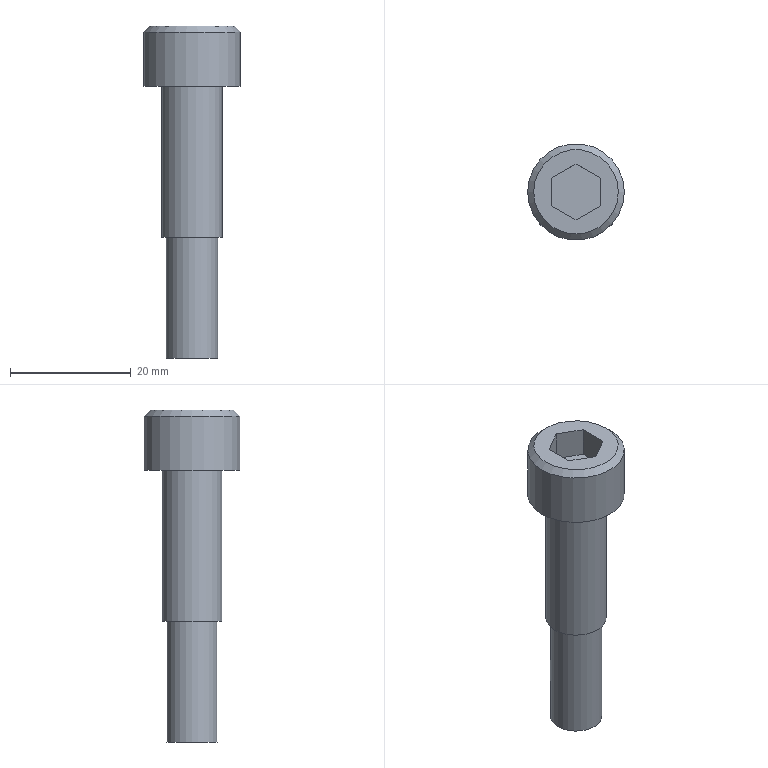Part | STEP file | M3-10_id42_x_t | 1 solid | 15 faces | box 16 x 16 x 55 mm | volume 4808 mm3 | plane 11 | cylinder 3 | cone 1 | commonest cylinder face diameters 8.5 x1 10 x1 16 x1
STEP:
#1=CARTESIAN_POINT('',(-209.8,-31.,-47.));
#2=VERTEX_POINT('',#1);
#3=CARTESIAN_POINT('',(-205.55,-31.,-47.));
#4=DIRECTION('',(0.,0.,-1.));
#5=DIRECTION('',(-1.,0.,0.));
#6=AXIS2_PLACEMENT_3D('',#3,#4,#5);
#7=CIRCLE('',#6,4.25);
#8=EDGE_CURVE('',#2,#2,#7,.T.);
#9=ORIENTED_EDGE('',*,*,#8,.F.);
#10=EDGE_LOOP('',(#9));
#11=FACE_BOUND('',#10,.T.);
#12=CARTESIAN_POINT('',(-200.55,-31.,-47.));
#13=VERTEX_POINT('',#12);
#14=CARTESIAN_POINT('',(-205.55,-31.,-47.));
#15=DIRECTION('',(0.,0.,1.));
#16=DIRECTION('',(1.,0.,0.));
#17=AXIS2_PLACEMENT_3D('',#14,#15,#16);
#18=CIRCLE('',#17,5.);
#19=EDGE_CURVE('',#13,#13,#18,.T.);
#20=ORIENTED_EDGE('',*,*,#19,.F.);
#21=EDGE_LOOP('',(#20));
#22=FACE_BOUND('',#21,.T.);
#23=CARTESIAN_POINT('',(-205.55,-31.,-47.));
#24=DIRECTION('',(0.,0.,-1.));
#25=DIRECTION('',(-1.,0.,0.));
#26=AXIS2_PLACEMENT_3D('',#23,#24,#25);
#27=PLANE('',#26);
#28=ADVANCED_FACE('',(#11,#22),#27,.T.);
#29=CARTESIAN_POINT('',(-210.55,-31.,-22.));
#30=VERTEX_POINT('',#29);
#31=CARTESIAN_POINT('',(-205.55,-31.,-22.));
#32=DIRECTION('',(0.,0.,1.));
#33=DIRECTION('',(-1.,0.,0.));
#34=AXIS2_PLACEMENT_3D('',#31,#32,#33);
#35=CIRCLE('',#34,5.);
#36=EDGE_CURVE('',#30,#30,#35,.T.);
#37=ORIENTED_EDGE('',*,*,#36,.F.);
#38=EDGE_LOOP('',(#37));
#39=FACE_BOUND('',#38,.T.);
#40=ORIENTED_EDGE('',*,*,#19,.T.);
#41=EDGE_LOOP('',(#40));
#42=FACE_BOUND('',#41,.T.);
#43=CARTESIAN_POINT('',(-205.55,-31.,-47.));
#44=DIRECTION('',(0.,0.,1.));
#45=DIRECTION('',(1.,0.,0.));
#46=AXIS2_PLACEMENT_3D('',#43,#44,#45);
#47=CYLINDRICAL_SURFACE('',#46,5.);
#48=ADVANCED_FACE('',(#39,#42),#47,.T.);
#49=CARTESIAN_POINT('',(-201.3,-31.,-67.));
#50=VERTEX_POINT('',#49);
#51=CARTESIAN_POINT('',(-205.55,-31.,-67.));
#52=DIRECTION('',(0.,0.,1.));
#53=DIRECTION('',(1.,0.,0.));
#54=AXIS2_PLACEMENT_3D('',#51,#52,#53);
#55=CIRCLE('',#54,4.25);
#56=EDGE_CURVE('',#50,#50,#55,.T.);
#57=ORIENTED_EDGE('',*,*,#56,.F.);
#58=EDGE_LOOP('',(#57));
#59=FACE_OUTER_BOUND('',#58,.T.);
#60=CARTESIAN_POINT('',(-205.55,-31.,-67.));
#61=DIRECTION('',(0.,0.,-1.));
#62=DIRECTION('',(-1.,0.,0.));
#63=AXIS2_PLACEMENT_3D('',#60,#61,#62);
#64=PLANE('',#63);
#65=ADVANCED_FACE('',(#59),#64,.T.);
#66=ORIENTED_EDGE('',*,*,#56,.T.);
#67=EDGE_LOOP('',(#66));
#68=FACE_BOUND('',#67,.T.);
#69=ORIENTED_EDGE('',*,*,#8,.T.);
#70=EDGE_LOOP('',(#69));
#71=FACE_BOUND('',#70,.T.);
#72=CARTESIAN_POINT('',(-205.55,-31.,-47.));
#73=DIRECTION('',(0.,0.,-1.));
#74=DIRECTION('',(1.,0.,0.));
#75=AXIS2_PLACEMENT_3D('',#72,#73,#74);
#76=CYLINDRICAL_SURFACE('',#75,4.25);
#77=ADVANCED_FACE('',(#68,#71),#76,.T.);
#78=CARTESIAN_POINT('',(-209.55,-28.691,-12.));
#79=VERTEX_POINT('',#78);
#80=CARTESIAN_POINT('',(-209.55,-33.309,-12.));
#81=VERTEX_POINT('',#80);
#82=CARTESIAN_POINT('',(-209.55,-28.691,-12.));
#83=DIRECTION('',(0.,-1.,0.));
#84=VECTOR('',#83,1.);
#85=LINE('',#82,#84);
#86=EDGE_CURVE('',#79,#81,#85,.T.);
#87=ORIENTED_EDGE('',*,*,#86,.F.);
#88=CARTESIAN_POINT('',(-205.55,-26.381,-12.));
#89=VERTEX_POINT('',#88);
#90=CARTESIAN_POINT('',(-205.55,-26.381,-12.));
#91=DIRECTION('',(-0.866,-0.5,0.));
#92=VECTOR('',#91,1.);
#93=LINE('',#90,#92);
#94=EDGE_CURVE('',#89,#79,#93,.T.);
#95=ORIENTED_EDGE('',*,*,#94,.F.);
#96=CARTESIAN_POINT('',(-201.55,-28.691,-12.));
#97=VERTEX_POINT('',#96);
#98=CARTESIAN_POINT('',(-201.55,-28.691,-12.));
#99=DIRECTION('',(-0.866,0.5,0.));
#100=VECTOR('',#99,1.);
#101=LINE('',#98,#100);
#102=EDGE_CURVE('',#97,#89,#101,.T.);
#103=ORIENTED_EDGE('',*,*,#102,.F.);
#104=CARTESIAN_POINT('',(-201.55,-33.309,-12.));
#105=VERTEX_POINT('',#104);
#106=CARTESIAN_POINT('',(-201.55,-33.309,-12.));
#107=DIRECTION('',(0.,1.,0.));
#108=VECTOR('',#107,1.);
#109=LINE('',#106,#108);
#110=EDGE_CURVE('',#105,#97,#109,.T.);
#111=ORIENTED_EDGE('',*,*,#110,.F.);
#112=CARTESIAN_POINT('',(-205.55,-35.619,-12.));
#113=VERTEX_POINT('',#112);
#114=CARTESIAN_POINT('',(-205.55,-35.619,-12.));
#115=DIRECTION('',(0.866,0.5,0.));
#116=VECTOR('',#115,1.);
#117=LINE('',#114,#116);
#118=EDGE_CURVE('',#113,#105,#117,.T.);
#119=ORIENTED_EDGE('',*,*,#118,.F.);
#120=CARTESIAN_POINT('',(-209.55,-33.309,-12.));
#121=DIRECTION('',(0.866,-0.5,0.));
#122=VECTOR('',#121,1.);
#123=LINE('',#120,#122);
#124=EDGE_CURVE('',#81,#113,#123,.T.);
#125=ORIENTED_EDGE('',*,*,#124,.F.);
#126=EDGE_LOOP('',(#87,#95,#103,#111,#119,#125));
#127=FACE_BOUND('',#126,.T.);
#128=CARTESIAN_POINT('',(-198.55,-31.,-12.));
#129=VERTEX_POINT('',#128);
#130=CARTESIAN_POINT('',(-205.55,-31.,-12.));
#131=DIRECTION('',(0.,0.,1.));
#132=DIRECTION('',(1.,0.,0.));
#133=AXIS2_PLACEMENT_3D('',#130,#131,#132);
#134=CIRCLE('',#133,7.);
#135=EDGE_CURVE('',#129,#129,#134,.T.);
#136=ORIENTED_EDGE('',*,*,#135,.T.);
#137=EDGE_LOOP('',(#136));
#138=FACE_BOUND('',#137,.T.);
#139=CARTESIAN_POINT('',(-205.55,-31.,-12.));
#140=DIRECTION('',(0.,0.,1.));
#141=DIRECTION('',(1.,0.,0.));
#142=AXIS2_PLACEMENT_3D('',#139,#140,#141);
#143=PLANE('',#142);
#144=ADVANCED_FACE('',(#127,#138),#143,.T.);
#145=ORIENTED_EDGE('',*,*,#36,.T.);
#146=EDGE_LOOP('',(#145));
#147=FACE_BOUND('',#146,.T.);
#148=CARTESIAN_POINT('',(-197.55,-31.,-22.));
#149=VERTEX_POINT('',#148);
#150=CARTESIAN_POINT('',(-205.55,-31.,-22.));
#151=DIRECTION('',(0.,0.,1.));
#152=DIRECTION('',(1.,0.,0.));
#153=AXIS2_PLACEMENT_3D('',#150,#151,#152);
#154=CIRCLE('',#153,8.);
#155=EDGE_CURVE('',#149,#149,#154,.T.);
#156=ORIENTED_EDGE('',*,*,#155,.F.);
#157=EDGE_LOOP('',(#156));
#158=FACE_BOUND('',#157,.T.);
#159=CARTESIAN_POINT('',(-205.55,-31.,-22.));
#160=DIRECTION('',(0.,0.,-1.));
#161=DIRECTION('',(-1.,0.,0.));
#162=AXIS2_PLACEMENT_3D('',#159,#160,#161);
#163=PLANE('',#162);
#164=ADVANCED_FACE('',(#147,#158),#163,.T.);
#165=CARTESIAN_POINT('',(-197.55,-31.,-13.));
#166=VERTEX_POINT('',#165);
#167=CARTESIAN_POINT('',(-205.55,-31.,-13.));
#168=DIRECTION('',(0.,0.,-1.));
#169=DIRECTION('',(1.,0.,0.));
#170=AXIS2_PLACEMENT_3D('',#167,#168,#169);
#171=CIRCLE('',#170,8.);
#172=EDGE_CURVE('',#166,#166,#171,.T.);
#173=ORIENTED_EDGE('',*,*,#172,.T.);
#174=EDGE_LOOP('',(#173));
#175=FACE_BOUND('',#174,.T.);
#176=ORIENTED_EDGE('',*,*,#155,.T.);
#177=EDGE_LOOP('',(#176));
#178=FACE_BOUND('',#177,.T.);
#179=CARTESIAN_POINT('',(-205.55,-31.,-22.));
#180=DIRECTION('',(0.,0.,1.));
#181=DIRECTION('',(1.,0.,0.));
#182=AXIS2_PLACEMENT_3D('',#179,#180,#181);
#183=CYLINDRICAL_SURFACE('',#182,8.);
#184=ADVANCED_FACE('',(#175,#178),#183,.T.);
#185=ORIENTED_EDGE('',*,*,#135,.F.);
#186=EDGE_LOOP('',(#185));
#187=FACE_BOUND('',#186,.T.);
#188=ORIENTED_EDGE('',*,*,#172,.F.);
#189=EDGE_LOOP('',(#188));
#190=FACE_BOUND('',#189,.T.);
#191=CARTESIAN_POINT('',(-205.55,-31.,-13.));
#192=DIRECTION('',(0.,0.,-1.));
#193=DIRECTION('',(-1.,0.,0.));
#194=AXIS2_PLACEMENT_3D('',#191,#192,#193);
#195=CONICAL_SURFACE('',#194,8.,45.);
#196=ADVANCED_FACE('',(#187,#190),#195,.T.);
#197=ORIENTED_EDGE('',*,*,#86,.T.);
#198=CARTESIAN_POINT('',(-209.55,-33.309,-17.));
#199=VERTEX_POINT('',#198);
#200=CARTESIAN_POINT('',(-209.55,-33.309,-17.));
#201=DIRECTION('',(0.,0.,-1.));
#202=VECTOR('',#201,1.);
#203=LINE('',#200,#202);
#204=EDGE_CURVE('',#81,#199,#203,.T.);
#205=ORIENTED_EDGE('',*,*,#204,.T.);
#206=CARTESIAN_POINT('',(-209.55,-28.691,-17.));
#207=VERTEX_POINT('',#206);
#208=CARTESIAN_POINT('',(-209.55,-28.691,-17.));
#209=DIRECTION('',(0.,1.,0.));
#210=VECTOR('',#209,1.);
#211=LINE('',#208,#210);
#212=EDGE_CURVE('',#199,#207,#211,.T.);
#213=ORIENTED_EDGE('',*,*,#212,.T.);
#214=CARTESIAN_POINT('',(-209.55,-28.691,-17.));
#215=DIRECTION('',(0.,0.,-1.));
#216=VECTOR('',#215,1.);
#217=LINE('',#214,#216);
#218=EDGE_CURVE('',#79,#207,#217,.T.);
#219=ORIENTED_EDGE('',*,*,#218,.F.);
#220=EDGE_LOOP('',(#197,#205,#213,#219));
#221=FACE_OUTER_BOUND('',#220,.T.);
#222=CARTESIAN_POINT('',(-209.55,-28.691,-17.));
#223=DIRECTION('',(-1.,0.,0.));
#224=DIRECTION('',(0.,-1.,0.));
#225=AXIS2_PLACEMENT_3D('',#222,#223,#224);
#226=PLANE('',#225);
#227=ADVANCED_FACE('',(#221),#226,.F.);
#228=ORIENTED_EDGE('',*,*,#124,.T.);
#229=CARTESIAN_POINT('',(-205.55,-35.619,-17.));
#230=VERTEX_POINT('',#229);
#231=CARTESIAN_POINT('',(-205.55,-35.619,-17.));
#232=DIRECTION('',(0.,0.,-1.));
#233=VECTOR('',#232,1.);
#234=LINE('',#231,#233);
#235=EDGE_CURVE('',#113,#230,#234,.T.);
#236=ORIENTED_EDGE('',*,*,#235,.T.);
#237=CARTESIAN_POINT('',(-209.55,-33.309,-17.));
#238=DIRECTION('',(-0.866,0.5,0.));
#239=VECTOR('',#238,1.);
#240=LINE('',#237,#239);
#241=EDGE_CURVE('',#230,#199,#240,.T.);
#242=ORIENTED_EDGE('',*,*,#241,.T.);
#243=ORIENTED_EDGE('',*,*,#204,.F.);
#244=EDGE_LOOP('',(#228,#236,#242,#243));
#245=FACE_OUTER_BOUND('',#244,.T.);
#246=CARTESIAN_POINT('',(-209.55,-33.309,-17.));
#247=DIRECTION('',(-0.5,-0.866,0.));
#248=DIRECTION('',(0.866,-0.5,0.));
#249=AXIS2_PLACEMENT_3D('',#246,#247,#248);
#250=PLANE('',#249);
#251=ADVANCED_FACE('',(#245),#250,.F.);
#252=ORIENTED_EDGE('',*,*,#118,.T.);
#253=CARTESIAN_POINT('',(-201.55,-33.309,-17.));
#254=VERTEX_POINT('',#253);
#255=CARTESIAN_POINT('',(-201.55,-33.309,-17.));
#256=DIRECTION('',(0.,0.,-1.));
#257=VECTOR('',#256,1.);
#258=LINE('',#255,#257);
#259=EDGE_CURVE('',#105,#254,#258,.T.);
#260=ORIENTED_EDGE('',*,*,#259,.T.);
#261=CARTESIAN_POINT('',(-205.55,-35.619,-17.));
#262=DIRECTION('',(-0.866,-0.5,0.));
#263=VECTOR('',#262,1.);
#264=LINE('',#261,#263);
#265=EDGE_CURVE('',#254,#230,#264,.T.);
#266=ORIENTED_EDGE('',*,*,#265,.T.);
#267=ORIENTED_EDGE('',*,*,#235,.F.);
#268=EDGE_LOOP('',(#252,#260,#266,#267));
#269=FACE_OUTER_BOUND('',#268,.T.);
#270=CARTESIAN_POINT('',(-205.55,-35.619,-17.));
#271=DIRECTION('',(0.5,-0.866,0.));
#272=DIRECTION('',(0.866,0.5,0.));
#273=AXIS2_PLACEMENT_3D('',#270,#271,#272);
#274=PLANE('',#273);
#275=ADVANCED_FACE('',(#269),#274,.F.);
#276=ORIENTED_EDGE('',*,*,#110,.T.);
#277=CARTESIAN_POINT('',(-201.55,-28.691,-17.));
#278=VERTEX_POINT('',#277);
#279=CARTESIAN_POINT('',(-201.55,-28.691,-17.));
#280=DIRECTION('',(0.,0.,-1.));
#281=VECTOR('',#280,1.);
#282=LINE('',#279,#281);
#283=EDGE_CURVE('',#97,#278,#282,.T.);
#284=ORIENTED_EDGE('',*,*,#283,.T.);
#285=CARTESIAN_POINT('',(-201.55,-33.309,-17.));
#286=DIRECTION('',(0.,-1.,0.));
#287=VECTOR('',#286,1.);
#288=LINE('',#285,#287);
#289=EDGE_CURVE('',#278,#254,#288,.T.);
#290=ORIENTED_EDGE('',*,*,#289,.T.);
#291=ORIENTED_EDGE('',*,*,#259,.F.);
#292=EDGE_LOOP('',(#276,#284,#290,#291));
#293=FACE_OUTER_BOUND('',#292,.T.);
#294=CARTESIAN_POINT('',(-201.55,-33.309,-17.));
#295=DIRECTION('',(1.,0.,0.));
#296=DIRECTION('',(0.,1.,0.));
#297=AXIS2_PLACEMENT_3D('',#294,#295,#296);
#298=PLANE('',#297);
#299=ADVANCED_FACE('',(#293),#298,.F.);
#300=ORIENTED_EDGE('',*,*,#102,.T.);
#301=CARTESIAN_POINT('',(-205.55,-26.381,-17.));
#302=VERTEX_POINT('',#301);
#303=CARTESIAN_POINT('',(-205.55,-26.381,-17.));
#304=DIRECTION('',(0.,0.,-1.));
#305=VECTOR('',#304,1.);
#306=LINE('',#303,#305);
#307=EDGE_CURVE('',#89,#302,#306,.T.);
#308=ORIENTED_EDGE('',*,*,#307,.T.);
#309=CARTESIAN_POINT('',(-201.55,-28.691,-17.));
#310=DIRECTION('',(0.866,-0.5,0.));
#311=VECTOR('',#310,1.);
#312=LINE('',#309,#311);
#313=EDGE_CURVE('',#302,#278,#312,.T.);
#314=ORIENTED_EDGE('',*,*,#313,.T.);
#315=ORIENTED_EDGE('',*,*,#283,.F.);
#316=EDGE_LOOP('',(#300,#308,#314,#315));
#317=FACE_OUTER_BOUND('',#316,.T.);
#318=CARTESIAN_POINT('',(-201.55,-28.691,-17.));
#319=DIRECTION('',(0.5,0.866,0.));
#320=DIRECTION('',(-0.866,0.5,0.));
#321=AXIS2_PLACEMENT_3D('',#318,#319,#320);
#322=PLANE('',#321);
#323=ADVANCED_FACE('',(#317),#322,.F.);
#324=ORIENTED_EDGE('',*,*,#94,.T.);
#325=ORIENTED_EDGE('',*,*,#218,.T.);
#326=CARTESIAN_POINT('',(-205.55,-26.381,-17.));
#327=DIRECTION('',(0.866,0.5,0.));
#328=VECTOR('',#327,1.);
#329=LINE('',#326,#328);
#330=EDGE_CURVE('',#207,#302,#329,.T.);
#331=ORIENTED_EDGE('',*,*,#330,.T.);
#332=ORIENTED_EDGE('',*,*,#307,.F.);
#333=EDGE_LOOP('',(#324,#325,#331,#332));
#334=FACE_OUTER_BOUND('',#333,.T.);
#335=CARTESIAN_POINT('',(-205.55,-26.381,-17.));
#336=DIRECTION('',(-0.5,0.866,0.));
#337=DIRECTION('',(-0.866,-0.5,0.));
#338=AXIS2_PLACEMENT_3D('',#335,#336,#337);
#339=PLANE('',#338);
#340=ADVANCED_FACE('',(#334),#339,.F.);
#341=ORIENTED_EDGE('',*,*,#212,.F.);
#342=ORIENTED_EDGE('',*,*,#241,.F.);
#343=ORIENTED_EDGE('',*,*,#265,.F.);
#344=ORIENTED_EDGE('',*,*,#289,.F.);
#345=ORIENTED_EDGE('',*,*,#313,.F.);
#346=ORIENTED_EDGE('',*,*,#330,.F.);
#347=EDGE_LOOP('',(#341,#342,#343,#344,#345,#346));
#348=FACE_OUTER_BOUND('',#347,.T.);
#349=CARTESIAN_POINT('',(-205.55,-31.,-17.));
#350=DIRECTION('',(0.,0.,1.));
#351=DIRECTION('',(1.,0.,0.));
#352=AXIS2_PLACEMENT_3D('',#349,#350,#351);
#353=PLANE('',#352);
#354=ADVANCED_FACE('',(#348),#353,.T.);
#355=CLOSED_SHELL('',(#28,#48,#65,#77,#144,#164,#184,#196,#227,#251,#275,#299,#323,#340,#354));
#356=MANIFOLD_SOLID_BREP('',#355);
#357=(LENGTH_UNIT()NAMED_UNIT(*)SI_UNIT(.MILLI.,.METRE.));
#358=UNCERTAINTY_MEASURE_WITH_UNIT(LENGTH_MEASURE(0.00002),#357,'','');
#359=(NAMED_UNIT(*)PLANE_ANGLE_UNIT()SI_UNIT($,.RADIAN.));
#360=PLANE_ANGLE_MEASURE_WITH_UNIT(PLANE_ANGLE_MEASURE(0.01745),#359);
#361=DIMENSIONAL_EXPONENTS(0.,0.,0.,0.,0.,0.,0.);
#362=(CONVERSION_BASED_UNIT('DEGREE',#360)NAMED_UNIT(#361)PLANE_ANGLE_UNIT());
#363=(NAMED_UNIT(*)SI_UNIT($,.STERADIAN.)SOLID_ANGLE_UNIT());
#364=(GEOMETRIC_REPRESENTATION_CONTEXT(3)GLOBAL_UNCERTAINTY_ASSIGNED_CONTEXT((#358))GLOBAL_UNIT_ASSIGNED_CONTEXT((#357,#362,#363))REPRESENTATION_CONTEXT('',''));
#365=ADVANCED_BREP_SHAPE_REPRESENTATION('',(#356),#364);